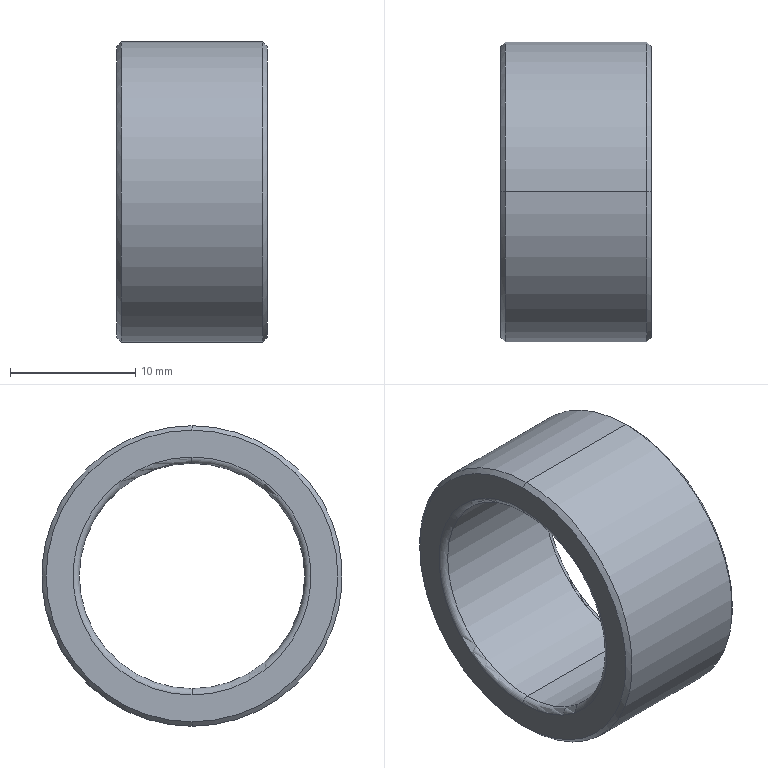Part | SolidWorks | features BaseBody 1 | 1 solid | 14 faces | box 12 x 24 x 24 mm | volume 2360 mm3 | cone 4 | cylinder 4 | torus 4 | plane 2 | commonest cylinder face diameters 18 x2 24 x2
STEP:
#1=CARTESIAN_POINT('',(0.,0.,-11.646));
#2=VERTEX_POINT('',#1);
#3=CARTESIAN_POINT('',(0.,0.,11.646));
#4=VERTEX_POINT('',#3);
#5=CARTESIAN_POINT('',(0.,0.,0.));
#6=DIRECTION('',(1.,0.,0.));
#7=DIRECTION('',(0.,0.,-1.));
#8=AXIS2_PLACEMENT_3D('',#5,#6,#7);
#9=CIRCLE('',#8,11.646);
#10=EDGE_CURVE('',#2,#4,#9,.T.);
#11=ORIENTED_EDGE('',*,*,#10,.T.);
#12=CARTESIAN_POINT('',(0.3536,0.,12.));
#13=VERTEX_POINT('',#12);
#14=CARTESIAN_POINT('',(0.3536,0.,12.));
#15=DIRECTION('',(0.7071,0.,0.7071));
#16=VECTOR('',#15,1000.);
#17=LINE('',#14,#16);
#18=EDGE_CURVE('',#4,#13,#17,.T.);
#19=ORIENTED_EDGE('',*,*,#18,.T.);
#20=CARTESIAN_POINT('',(0.3536,0.,-12.));
#21=VERTEX_POINT('',#20);
#22=CARTESIAN_POINT('',(0.3536,0.,0.));
#23=DIRECTION('',(1.,0.,0.));
#24=DIRECTION('',(0.,0.,-1.));
#25=AXIS2_PLACEMENT_3D('',#22,#23,#24);
#26=CIRCLE('',#25,12.);
#27=EDGE_CURVE('',#21,#13,#26,.T.);
#28=ORIENTED_EDGE('',*,*,#27,.F.);
#29=CARTESIAN_POINT('',(0.3536,0.,-12.));
#30=DIRECTION('',(0.7071,0.,-0.7071));
#31=VECTOR('',#30,1000.);
#32=LINE('',#29,#31);
#33=EDGE_CURVE('',#2,#21,#32,.T.);
#34=ORIENTED_EDGE('',*,*,#33,.F.);
#35=EDGE_LOOP('',(#11,#19,#28,#34));
#36=FACE_OUTER_BOUND('',#35,.T.);
#37=CARTESIAN_POINT('',(0.3536,0.,0.));
#38=DIRECTION('',(1.,0.,0.));
#39=DIRECTION('',(0.,0.,-1.));
#40=AXIS2_PLACEMENT_3D('',#37,#38,#39);
#41=CONICAL_SURFACE('',#40,12.,0.7854);
#42=ADVANCED_FACE('',(#36),#41,.T.);
#43=CARTESIAN_POINT('',(11.646,0.,12.));
#44=VERTEX_POINT('',#43);
#45=CARTESIAN_POINT('',(11.646,0.,-12.));
#46=VERTEX_POINT('',#45);
#47=CARTESIAN_POINT('',(11.646,0.,0.));
#48=DIRECTION('',(1.,0.,0.));
#49=DIRECTION('',(0.,0.,-1.));
#50=AXIS2_PLACEMENT_3D('',#47,#48,#49);
#51=CIRCLE('',#50,12.);
#52=EDGE_CURVE('',#44,#46,#51,.T.);
#53=ORIENTED_EDGE('',*,*,#52,.F.);
#54=CARTESIAN_POINT('',(12.,0.,12.));
#55=DIRECTION('',(-1.,0.,0.));
#56=VECTOR('',#55,1000.);
#57=LINE('',#54,#56);
#58=EDGE_CURVE('',#44,#13,#57,.T.);
#59=ORIENTED_EDGE('',*,*,#58,.T.);
#60=CARTESIAN_POINT('',(0.3536,0.,0.));
#61=DIRECTION('',(1.,0.,0.));
#62=DIRECTION('',(0.,0.,-1.));
#63=AXIS2_PLACEMENT_3D('',#60,#61,#62);
#64=CIRCLE('',#63,12.);
#65=EDGE_CURVE('',#13,#21,#64,.T.);
#66=ORIENTED_EDGE('',*,*,#65,.T.);
#67=CARTESIAN_POINT('',(12.,0.,-12.));
#68=DIRECTION('',(-1.,0.,0.));
#69=VECTOR('',#68,1000.);
#70=LINE('',#67,#69);
#71=EDGE_CURVE('',#46,#21,#70,.T.);
#72=ORIENTED_EDGE('',*,*,#71,.F.);
#73=EDGE_LOOP('',(#53,#59,#66,#72));
#74=FACE_OUTER_BOUND('',#73,.T.);
#75=CARTESIAN_POINT('',(12.,0.,0.));
#76=DIRECTION('',(-1.,0.,0.));
#77=DIRECTION('',(0.,0.,-1.));
#78=AXIS2_PLACEMENT_3D('',#75,#76,#77);
#79=CYLINDRICAL_SURFACE('',#78,12.);
#80=ADVANCED_FACE('',(#74),#79,.T.);
#81=CARTESIAN_POINT('',(12.,0.,-11.646));
#82=VERTEX_POINT('',#81);
#83=CARTESIAN_POINT('',(12.,0.,11.646));
#84=VERTEX_POINT('',#83);
#85=CARTESIAN_POINT('',(12.,0.,0.));
#86=DIRECTION('',(1.,0.,0.));
#87=DIRECTION('',(0.,0.,-1.));
#88=AXIS2_PLACEMENT_3D('',#85,#86,#87);
#89=CIRCLE('',#88,11.646);
#90=EDGE_CURVE('',#82,#84,#89,.T.);
#91=ORIENTED_EDGE('',*,*,#90,.F.);
#92=CARTESIAN_POINT('',(12.,0.,-11.646));
#93=DIRECTION('',(-0.7071,0.,-0.7071));
#94=VECTOR('',#93,1000.);
#95=LINE('',#92,#94);
#96=EDGE_CURVE('',#82,#46,#95,.T.);
#97=ORIENTED_EDGE('',*,*,#96,.T.);
#98=CARTESIAN_POINT('',(11.646,0.,0.));
#99=DIRECTION('',(1.,0.,0.));
#100=DIRECTION('',(0.,0.,-1.));
#101=AXIS2_PLACEMENT_3D('',#98,#99,#100);
#102=CIRCLE('',#101,12.);
#103=EDGE_CURVE('',#46,#44,#102,.T.);
#104=ORIENTED_EDGE('',*,*,#103,.T.);
#105=CARTESIAN_POINT('',(12.,0.,11.646));
#106=DIRECTION('',(-0.7071,0.,0.7071));
#107=VECTOR('',#106,1000.);
#108=LINE('',#105,#107);
#109=EDGE_CURVE('',#84,#44,#108,.T.);
#110=ORIENTED_EDGE('',*,*,#109,.F.);
#111=EDGE_LOOP('',(#91,#97,#104,#110));
#112=FACE_OUTER_BOUND('',#111,.T.);
#113=CARTESIAN_POINT('',(12.,0.,0.));
#114=DIRECTION('',(-1.,0.,0.));
#115=DIRECTION('',(0.,0.,1.));
#116=AXIS2_PLACEMENT_3D('',#113,#114,#115);
#117=CONICAL_SURFACE('',#116,11.646,0.7854);
#118=ADVANCED_FACE('',(#112),#117,.T.);
#119=CARTESIAN_POINT('',(12.,0.,-9.5));
#120=VERTEX_POINT('',#119);
#121=CARTESIAN_POINT('',(12.,0.,9.5));
#122=VERTEX_POINT('',#121);
#123=CARTESIAN_POINT('',(12.,0.,0.));
#124=DIRECTION('',(1.,0.,0.));
#125=DIRECTION('',(0.,0.,-1.));
#126=AXIS2_PLACEMENT_3D('',#123,#124,#125);
#127=CIRCLE('',#126,9.5);
#128=EDGE_CURVE('',#120,#122,#127,.T.);
#129=ORIENTED_EDGE('',*,*,#128,.T.);
#130=CARTESIAN_POINT('',(11.5,0.,9.));
#131=VERTEX_POINT('',#130);
#132=CARTESIAN_POINT('',(11.5,0.,9.5));
#133=DIRECTION('',(0.,1.,0.));
#134=DIRECTION('',(0.,0.,1.));
#135=AXIS2_PLACEMENT_3D('',#132,#133,#134);
#136=CIRCLE('',#135,0.5);
#137=EDGE_CURVE('',#122,#131,#136,.T.);
#138=ORIENTED_EDGE('',*,*,#137,.T.);
#139=CARTESIAN_POINT('',(11.5,0.,-9.));
#140=VERTEX_POINT('',#139);
#141=CARTESIAN_POINT('',(11.5,0.,0.));
#142=DIRECTION('',(1.,0.,0.));
#143=DIRECTION('',(0.,0.,-1.));
#144=AXIS2_PLACEMENT_3D('',#141,#142,#143);
#145=CIRCLE('',#144,9.);
#146=EDGE_CURVE('',#140,#131,#145,.T.);
#147=ORIENTED_EDGE('',*,*,#146,.F.);
#148=CARTESIAN_POINT('',(11.5,0.,-9.5));
#149=DIRECTION('',(0.,-1.,0.));
#150=DIRECTION('',(0.,0.,-1.));
#151=AXIS2_PLACEMENT_3D('',#148,#149,#150);
#152=CIRCLE('',#151,0.5);
#153=EDGE_CURVE('',#120,#140,#152,.T.);
#154=ORIENTED_EDGE('',*,*,#153,.F.);
#155=EDGE_LOOP('',(#129,#138,#147,#154));
#156=FACE_OUTER_BOUND('',#155,.T.);
#157=CARTESIAN_POINT('',(11.5,0.,0.));
#158=DIRECTION('',(1.,0.,0.));
#159=DIRECTION('',(0.,0.,-1.));
#160=AXIS2_PLACEMENT_3D('',#157,#158,#159);
#161=TOROIDAL_SURFACE('',#160,9.5,0.5);
#162=ADVANCED_FACE('',(#156),#161,.T.);
#163=ORIENTED_EDGE('',*,*,#146,.T.);
#164=CARTESIAN_POINT('',(0.5,0.,9.));
#165=VERTEX_POINT('',#164);
#166=CARTESIAN_POINT('',(12.,0.,9.));
#167=DIRECTION('',(-1.,0.,0.));
#168=VECTOR('',#167,1000.);
#169=LINE('',#166,#168);
#170=EDGE_CURVE('',#131,#165,#169,.T.);
#171=ORIENTED_EDGE('',*,*,#170,.T.);
#172=CARTESIAN_POINT('',(0.5,0.,-9.));
#173=VERTEX_POINT('',#172);
#174=CARTESIAN_POINT('',(0.5,0.,0.));
#175=DIRECTION('',(1.,0.,0.));
#176=DIRECTION('',(0.,0.,-1.));
#177=AXIS2_PLACEMENT_3D('',#174,#175,#176);
#178=CIRCLE('',#177,9.);
#179=EDGE_CURVE('',#173,#165,#178,.T.);
#180=ORIENTED_EDGE('',*,*,#179,.F.);
#181=CARTESIAN_POINT('',(12.,0.,-9.));
#182=DIRECTION('',(-1.,0.,0.));
#183=VECTOR('',#182,1000.);
#184=LINE('',#181,#183);
#185=EDGE_CURVE('',#140,#173,#184,.T.);
#186=ORIENTED_EDGE('',*,*,#185,.F.);
#187=EDGE_LOOP('',(#163,#171,#180,#186));
#188=FACE_OUTER_BOUND('',#187,.T.);
#189=CARTESIAN_POINT('',(12.,0.,0.));
#190=DIRECTION('',(-1.,0.,0.));
#191=DIRECTION('',(0.,0.,-1.));
#192=AXIS2_PLACEMENT_3D('',#189,#190,#191);
#193=CYLINDRICAL_SURFACE('',#192,9.);
#194=ADVANCED_FACE('',(#188),#193,.F.);
#195=ORIENTED_EDGE('',*,*,#179,.T.);
#196=CARTESIAN_POINT('',(0.,0.,9.5));
#197=VERTEX_POINT('',#196);
#198=CARTESIAN_POINT('',(0.5,0.,9.5));
#199=DIRECTION('',(0.,1.,0.));
#200=DIRECTION('',(0.,0.,1.));
#201=AXIS2_PLACEMENT_3D('',#198,#199,#200);
#202=CIRCLE('',#201,0.5);
#203=EDGE_CURVE('',#165,#197,#202,.T.);
#204=ORIENTED_EDGE('',*,*,#203,.T.);
#205=CARTESIAN_POINT('',(0.,0.,-9.5));
#206=VERTEX_POINT('',#205);
#207=CARTESIAN_POINT('',(0.,0.,0.));
#208=DIRECTION('',(1.,0.,0.));
#209=DIRECTION('',(0.,0.,-1.));
#210=AXIS2_PLACEMENT_3D('',#207,#208,#209);
#211=CIRCLE('',#210,9.5);
#212=EDGE_CURVE('',#206,#197,#211,.T.);
#213=ORIENTED_EDGE('',*,*,#212,.F.);
#214=CARTESIAN_POINT('',(0.5,0.,-9.5));
#215=DIRECTION('',(0.,-1.,0.));
#216=DIRECTION('',(0.,0.,-1.));
#217=AXIS2_PLACEMENT_3D('',#214,#215,#216);
#218=CIRCLE('',#217,0.5);
#219=EDGE_CURVE('',#173,#206,#218,.T.);
#220=ORIENTED_EDGE('',*,*,#219,.F.);
#221=EDGE_LOOP('',(#195,#204,#213,#220));
#222=FACE_OUTER_BOUND('',#221,.T.);
#223=CARTESIAN_POINT('',(0.5,0.,0.));
#224=DIRECTION('',(1.,0.,0.));
#225=DIRECTION('',(0.,0.,-1.));
#226=AXIS2_PLACEMENT_3D('',#223,#224,#225);
#227=TOROIDAL_SURFACE('',#226,9.5,0.5);
#228=ADVANCED_FACE('',(#222),#227,.T.);
#229=ORIENTED_EDGE('',*,*,#10,.F.);
#230=CARTESIAN_POINT('',(0.,0.,0.));
#231=DIRECTION('',(1.,0.,0.));
#232=DIRECTION('',(0.,0.,-1.));
#233=AXIS2_PLACEMENT_3D('',#230,#231,#232);
#234=CIRCLE('',#233,11.646);
#235=EDGE_CURVE('',#4,#2,#234,.T.);
#236=ORIENTED_EDGE('',*,*,#235,.F.);
#237=EDGE_LOOP('',(#229,#236));
#238=FACE_OUTER_BOUND('',#237,.T.);
#239=ORIENTED_EDGE('',*,*,#212,.T.);
#240=CARTESIAN_POINT('',(0.,0.,0.));
#241=DIRECTION('',(1.,0.,0.));
#242=DIRECTION('',(0.,0.,-1.));
#243=AXIS2_PLACEMENT_3D('',#240,#241,#242);
#244=CIRCLE('',#243,9.5);
#245=EDGE_CURVE('',#197,#206,#244,.T.);
#246=ORIENTED_EDGE('',*,*,#245,.T.);
#247=EDGE_LOOP('',(#239,#246));
#248=FACE_BOUND('',#247,.T.);
#249=CARTESIAN_POINT('',(0.,11.646,0.));
#250=DIRECTION('',(-1.,0.,0.));
#251=DIRECTION('',(0.,0.,1.));
#252=AXIS2_PLACEMENT_3D('',#249,#250,#251);
#253=PLANE('',#252);
#254=ADVANCED_FACE('',(#238,#248),#253,.T.);
#255=ORIENTED_EDGE('',*,*,#203,.F.);
#256=CARTESIAN_POINT('',(0.5,0.,0.));
#257=DIRECTION('',(1.,0.,0.));
#258=DIRECTION('',(0.,0.,-1.));
#259=AXIS2_PLACEMENT_3D('',#256,#257,#258);
#260=CIRCLE('',#259,9.);
#261=EDGE_CURVE('',#165,#173,#260,.T.);
#262=ORIENTED_EDGE('',*,*,#261,.T.);
#263=ORIENTED_EDGE('',*,*,#219,.T.);
#264=ORIENTED_EDGE('',*,*,#245,.F.);
#265=EDGE_LOOP('',(#255,#262,#263,#264));
#266=FACE_OUTER_BOUND('',#265,.T.);
#267=CARTESIAN_POINT('',(0.5,0.,0.));
#268=DIRECTION('',(1.,0.,0.));
#269=DIRECTION('',(0.,0.,-1.));
#270=AXIS2_PLACEMENT_3D('',#267,#268,#269);
#271=TOROIDAL_SURFACE('',#270,9.5,0.5);
#272=ADVANCED_FACE('',(#266),#271,.T.);
#273=ORIENTED_EDGE('',*,*,#170,.F.);
#274=CARTESIAN_POINT('',(11.5,0.,0.));
#275=DIRECTION('',(1.,0.,0.));
#276=DIRECTION('',(0.,0.,-1.));
#277=AXIS2_PLACEMENT_3D('',#274,#275,#276);
#278=CIRCLE('',#277,9.);
#279=EDGE_CURVE('',#131,#140,#278,.T.);
#280=ORIENTED_EDGE('',*,*,#279,.T.);
#281=ORIENTED_EDGE('',*,*,#185,.T.);
#282=ORIENTED_EDGE('',*,*,#261,.F.);
#283=EDGE_LOOP('',(#273,#280,#281,#282));
#284=FACE_OUTER_BOUND('',#283,.T.);
#285=CARTESIAN_POINT('',(12.,0.,0.));
#286=DIRECTION('',(-1.,0.,0.));
#287=DIRECTION('',(0.,0.,-1.));
#288=AXIS2_PLACEMENT_3D('',#285,#286,#287);
#289=CYLINDRICAL_SURFACE('',#288,9.);
#290=ADVANCED_FACE('',(#284),#289,.F.);
#291=ORIENTED_EDGE('',*,*,#137,.F.);
#292=CARTESIAN_POINT('',(12.,0.,0.));
#293=DIRECTION('',(1.,0.,0.));
#294=DIRECTION('',(0.,0.,-1.));
#295=AXIS2_PLACEMENT_3D('',#292,#293,#294);
#296=CIRCLE('',#295,9.5);
#297=EDGE_CURVE('',#122,#120,#296,.T.);
#298=ORIENTED_EDGE('',*,*,#297,.T.);
#299=ORIENTED_EDGE('',*,*,#153,.T.);
#300=ORIENTED_EDGE('',*,*,#279,.F.);
#301=EDGE_LOOP('',(#291,#298,#299,#300));
#302=FACE_OUTER_BOUND('',#301,.T.);
#303=CARTESIAN_POINT('',(11.5,0.,0.));
#304=DIRECTION('',(1.,0.,0.));
#305=DIRECTION('',(0.,0.,-1.));
#306=AXIS2_PLACEMENT_3D('',#303,#304,#305);
#307=TOROIDAL_SURFACE('',#306,9.5,0.5);
#308=ADVANCED_FACE('',(#302),#307,.T.);
#309=CARTESIAN_POINT('',(12.,0.,0.));
#310=DIRECTION('',(1.,0.,0.));
#311=DIRECTION('',(0.,0.,-1.));
#312=AXIS2_PLACEMENT_3D('',#309,#310,#311);
#313=CIRCLE('',#312,11.646);
#314=EDGE_CURVE('',#84,#82,#313,.T.);
#315=ORIENTED_EDGE('',*,*,#314,.T.);
#316=ORIENTED_EDGE('',*,*,#90,.T.);
#317=EDGE_LOOP('',(#315,#316));
#318=FACE_OUTER_BOUND('',#317,.T.);
#319=ORIENTED_EDGE('',*,*,#128,.F.);
#320=ORIENTED_EDGE('',*,*,#297,.F.);
#321=EDGE_LOOP('',(#319,#320));
#322=FACE_BOUND('',#321,.T.);
#323=CARTESIAN_POINT('',(12.,9.5,0.));
#324=DIRECTION('',(1.,0.,0.));
#325=DIRECTION('',(0.,1.,0.));
#326=AXIS2_PLACEMENT_3D('',#323,#324,#325);
#327=PLANE('',#326);
#328=ADVANCED_FACE('',(#318,#322),#327,.T.);
#329=ORIENTED_EDGE('',*,*,#96,.F.);
#330=ORIENTED_EDGE('',*,*,#314,.F.);
#331=ORIENTED_EDGE('',*,*,#109,.T.);
#332=ORIENTED_EDGE('',*,*,#52,.T.);
#333=EDGE_LOOP('',(#329,#330,#331,#332));
#334=FACE_OUTER_BOUND('',#333,.T.);
#335=CARTESIAN_POINT('',(12.,0.,0.));
#336=DIRECTION('',(-1.,0.,0.));
#337=DIRECTION('',(0.,0.,1.));
#338=AXIS2_PLACEMENT_3D('',#335,#336,#337);
#339=CONICAL_SURFACE('',#338,11.646,0.7854);
#340=ADVANCED_FACE('',(#334),#339,.T.);
#341=ORIENTED_EDGE('',*,*,#58,.F.);
#342=ORIENTED_EDGE('',*,*,#103,.F.);
#343=ORIENTED_EDGE('',*,*,#71,.T.);
#344=ORIENTED_EDGE('',*,*,#27,.T.);
#345=EDGE_LOOP('',(#341,#342,#343,#344));
#346=FACE_OUTER_BOUND('',#345,.T.);
#347=CARTESIAN_POINT('',(12.,0.,0.));
#348=DIRECTION('',(-1.,0.,0.));
#349=DIRECTION('',(0.,0.,-1.));
#350=AXIS2_PLACEMENT_3D('',#347,#348,#349);
#351=CYLINDRICAL_SURFACE('',#350,12.);
#352=ADVANCED_FACE('',(#346),#351,.T.);
#353=ORIENTED_EDGE('',*,*,#18,.F.);
#354=ORIENTED_EDGE('',*,*,#235,.T.);
#355=ORIENTED_EDGE('',*,*,#33,.T.);
#356=ORIENTED_EDGE('',*,*,#65,.F.);
#357=EDGE_LOOP('',(#353,#354,#355,#356));
#358=FACE_OUTER_BOUND('',#357,.T.);
#359=CARTESIAN_POINT('',(0.3536,0.,0.));
#360=DIRECTION('',(1.,0.,0.));
#361=DIRECTION('',(0.,0.,-1.));
#362=AXIS2_PLACEMENT_3D('',#359,#360,#361);
#363=CONICAL_SURFACE('',#362,12.,0.7854);
#364=ADVANCED_FACE('',(#358),#363,.T.);
#365=CLOSED_SHELL('',(#42,#80,#118,#162,#194,#228,#254,#272,#290,#308,#328,#340,#352,#364));
#366=MANIFOLD_SOLID_BREP('',#365);
#367=CARTESIAN_POINT('',(0.,0.,0.));
#368=DIRECTION('',(0.,0.,1.));
#369=DIRECTION('',(1.,0.,0.));
#370=AXIS2_PLACEMENT_3D('',#367,#368,#369);
#371=(LENGTH_UNIT()NAMED_UNIT(*)SI_UNIT(.MILLI.,.METRE.));
#372=UNCERTAINTY_MEASURE_WITH_UNIT(LENGTH_MEASURE(0.00001),#371,'','');
#373=(NAMED_UNIT(*)PLANE_ANGLE_UNIT()SI_UNIT($,.RADIAN.));
#374=(NAMED_UNIT(*)SI_UNIT($,.STERADIAN.)SOLID_ANGLE_UNIT());
#375=(GEOMETRIC_REPRESENTATION_CONTEXT(3)GLOBAL_UNCERTAINTY_ASSIGNED_CONTEXT((#372))GLOBAL_UNIT_ASSIGNED_CONTEXT((#371,#373,#374))REPRESENTATION_CONTEXT('',''));
#376=ADVANCED_BREP_SHAPE_REPRESENTATION('',(#366,#370),#375);